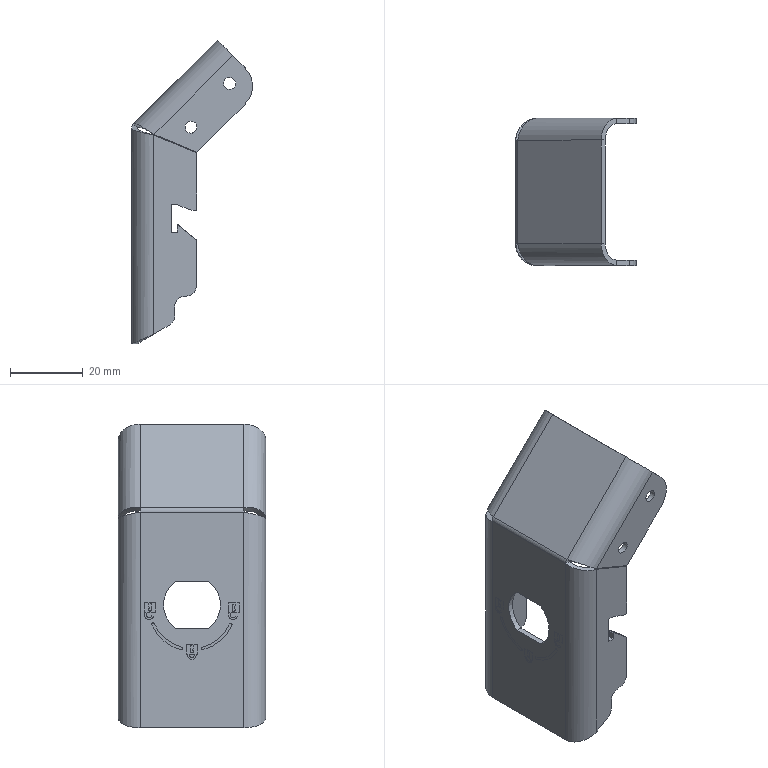Part | SolidWorks | features BaseBody 1 | 1 solid | 97 faces | box 33.223 x 40.533 x 83.47 mm | volume 8300 mm3 | plane 55 | cylinder 36 | spline 6 | commonest cylinder face diameters 3.3 x8 6 x6 1 x4 9 x4 12 x4 0.4 x3